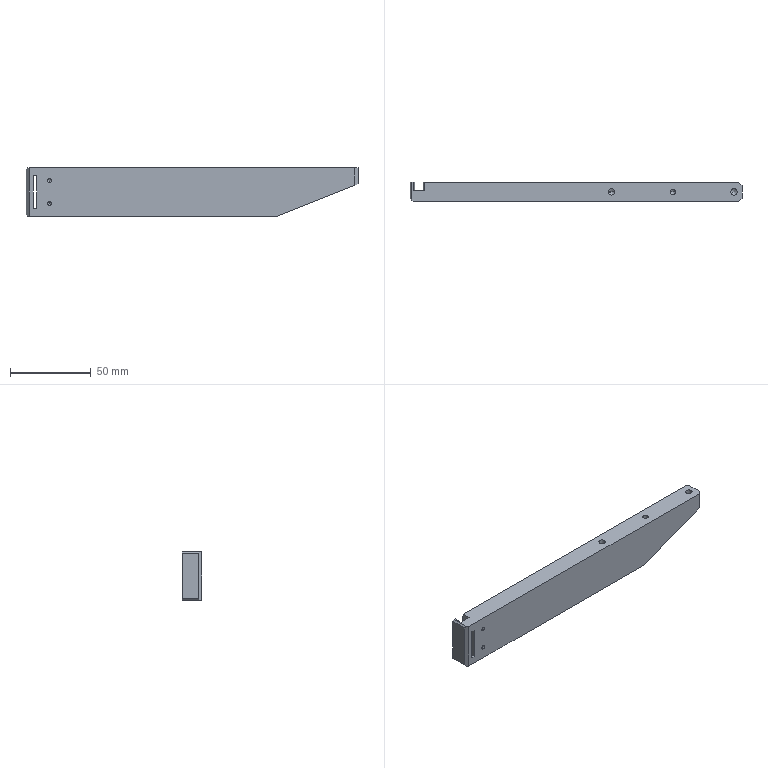Part | STEP file | QA-FB06 | 1 solid | 42 faces | box 206 x 12 x 30 mm | volume 66556 mm3 | plane 22 | cylinder 10 | cone 10 | commonest cylinder face diameters 2.5 x4 4 x4 3.3 x2